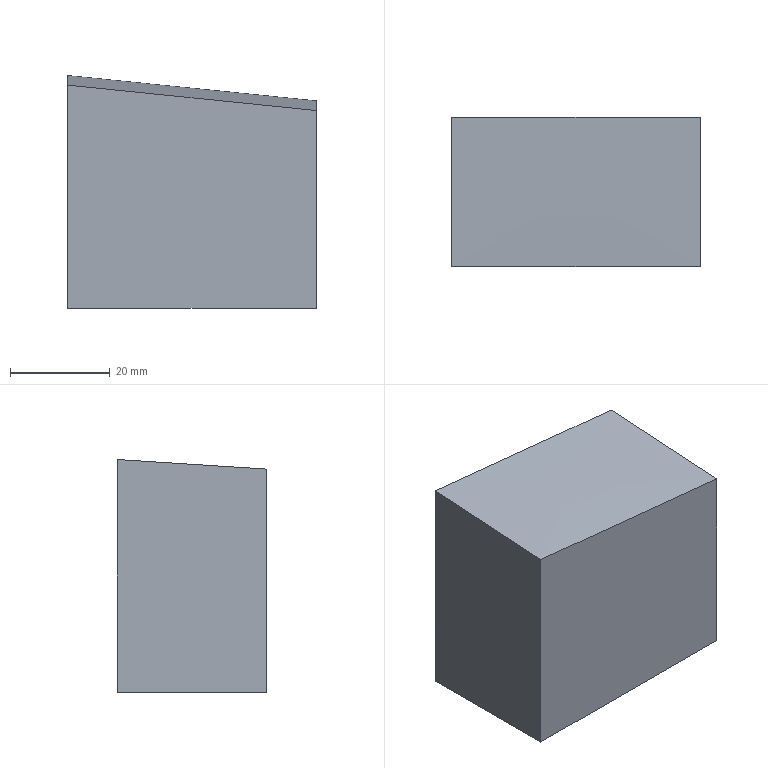Part | NX | features solid 2 | 1 solid | 6 faces | box 50 x 30 x 46.829 mm | volume 65041 mm3 | plane 5 | spline 1
STEP:
#1=CARTESIAN_POINT('',(437.5,-295.,54.902));
#2=VERTEX_POINT('',#1);
#3=CARTESIAN_POINT('',(487.5,-295.,49.786));
#4=VERTEX_POINT('',#3);
#5=CARTESIAN_POINT('',(437.5,-295.,54.902));
#6=CARTESIAN_POINT('',(454.172,-295.,53.249));
#7=CARTESIAN_POINT('',(470.839,-295.,51.542));
#8=CARTESIAN_POINT('',(487.5,-295.,49.786));
#9=B_SPLINE_CURVE_WITH_KNOTS('',3,(#5,#6,#7,#8),.UNSPECIFIED.,.F.,.F.,(4,4),(0.,0.05026),.UNSPECIFIED.);
#10=EDGE_CURVE('',#2,#4,#9,.T.);
#11=ORIENTED_EDGE('',*,*,#10,.F.);
#12=CARTESIAN_POINT('',(437.5,-295.,10.));
#13=VERTEX_POINT('',#12);
#14=CARTESIAN_POINT('',(437.5,-295.,210.));
#15=DIRECTION('',(0.,0.,-1.));
#16=VECTOR('',#15,1000.);
#17=LINE('',#14,#16);
#18=EDGE_CURVE('',#2,#13,#17,.T.);
#19=ORIENTED_EDGE('',*,*,#18,.T.);
#20=CARTESIAN_POINT('',(487.5,-295.,10.));
#21=VERTEX_POINT('',#20);
#22=CARTESIAN_POINT('',(437.5,-295.,10.));
#23=DIRECTION('',(1.,0.,0.));
#24=VECTOR('',#23,1000.);
#25=LINE('',#22,#24);
#26=EDGE_CURVE('',#13,#21,#25,.T.);
#27=ORIENTED_EDGE('',*,*,#26,.T.);
#28=CARTESIAN_POINT('',(487.5,-295.,210.));
#29=DIRECTION('',(0.,0.,-1.));
#30=VECTOR('',#29,1000.);
#31=LINE('',#28,#30);
#32=EDGE_CURVE('',#4,#21,#31,.T.);
#33=ORIENTED_EDGE('',*,*,#32,.F.);
#34=EDGE_LOOP('',(#11,#19,#27,#33));
#35=FACE_BOUND('',#34,.T.);
#36=CARTESIAN_POINT('',(437.5,-295.,210.));
#37=DIRECTION('',(0.,1.,0.));
#38=DIRECTION('',(0.,0.,1.));
#39=AXIS2_PLACEMENT_3D('',#36,#37,#38);
#40=PLANE('',#39);
#41=ADVANCED_FACE('',(#35),#40,.F.);
#42=ORIENTED_EDGE('',*,*,#18,.F.);
#43=CARTESIAN_POINT('',(437.5,-265.,56.829));
#44=VERTEX_POINT('',#43);
#45=CARTESIAN_POINT('',(437.5,-295.,54.902));
#46=CARTESIAN_POINT('',(437.5,-285.004,55.594));
#47=CARTESIAN_POINT('',(437.5,-275.003,56.235));
#48=CARTESIAN_POINT('',(437.5,-265.,56.829));
#49=B_SPLINE_CURVE_WITH_KNOTS('',3,(#45,#46,#47,#48),.UNSPECIFIED.,.F.,.F.,(4,4),(0.04695,0.07702),.UNSPECIFIED.);
#50=EDGE_CURVE('',#2,#44,#49,.T.);
#51=ORIENTED_EDGE('',*,*,#50,.T.);
#52=CARTESIAN_POINT('',(437.5,-265.,10.));
#53=VERTEX_POINT('',#52);
#54=CARTESIAN_POINT('',(437.5,-265.,210.));
#55=DIRECTION('',(0.,0.,-1.));
#56=VECTOR('',#55,1000.);
#57=LINE('',#54,#56);
#58=EDGE_CURVE('',#44,#53,#57,.T.);
#59=ORIENTED_EDGE('',*,*,#58,.T.);
#60=CARTESIAN_POINT('',(437.5,-515.,10.));
#61=DIRECTION('',(0.,-1.,0.));
#62=VECTOR('',#61,1000.);
#63=LINE('',#60,#62);
#64=EDGE_CURVE('',#13,#53,#63,.F.);
#65=ORIENTED_EDGE('',*,*,#64,.F.);
#66=EDGE_LOOP('',(#42,#51,#59,#65));
#67=FACE_BOUND('',#66,.T.);
#68=CARTESIAN_POINT('',(437.5,-515.,210.));
#69=DIRECTION('',(-1.,0.,0.));
#70=DIRECTION('',(0.,0.,1.));
#71=AXIS2_PLACEMENT_3D('',#68,#69,#70);
#72=PLANE('',#71);
#73=ADVANCED_FACE('',(#67),#72,.T.);
#74=ORIENTED_EDGE('',*,*,#58,.F.);
#75=CARTESIAN_POINT('',(487.5,-265.,51.724));
#76=VERTEX_POINT('',#75);
#77=CARTESIAN_POINT('',(437.5,-265.,56.829));
#78=CARTESIAN_POINT('',(454.171,-265.,55.18));
#79=CARTESIAN_POINT('',(470.839,-265.,53.476));
#80=CARTESIAN_POINT('',(487.5,-265.,51.724));
#81=B_SPLINE_CURVE_WITH_KNOTS('',3,(#77,#78,#79,#80),.UNSPECIFIED.,.F.,.F.,(4,4),(0.2849,0.3352),.UNSPECIFIED.);
#82=EDGE_CURVE('',#44,#76,#81,.T.);
#83=ORIENTED_EDGE('',*,*,#82,.T.);
#84=CARTESIAN_POINT('',(487.5,-265.,10.));
#85=VERTEX_POINT('',#84);
#86=CARTESIAN_POINT('',(487.5,-265.,210.));
#87=DIRECTION('',(0.,0.,-1.));
#88=VECTOR('',#87,1000.);
#89=LINE('',#86,#88);
#90=EDGE_CURVE('',#76,#85,#89,.T.);
#91=ORIENTED_EDGE('',*,*,#90,.T.);
#92=CARTESIAN_POINT('',(255.,-265.,10.));
#93=DIRECTION('',(-1.,0.,0.));
#94=VECTOR('',#93,1000.);
#95=LINE('',#92,#94);
#96=EDGE_CURVE('',#53,#85,#95,.F.);
#97=ORIENTED_EDGE('',*,*,#96,.F.);
#98=EDGE_LOOP('',(#74,#83,#91,#97));
#99=FACE_BOUND('',#98,.T.);
#100=CARTESIAN_POINT('',(255.,-265.,210.));
#101=DIRECTION('',(0.,1.,0.));
#102=DIRECTION('',(0.,0.,1.));
#103=AXIS2_PLACEMENT_3D('',#100,#101,#102);
#104=PLANE('',#103);
#105=ADVANCED_FACE('',(#99),#104,.T.);
#106=CARTESIAN_POINT('',(487.5,-295.,49.786));
#107=CARTESIAN_POINT('',(487.5,-285.005,50.482));
#108=CARTESIAN_POINT('',(487.5,-275.003,51.126));
#109=CARTESIAN_POINT('',(487.5,-265.,51.724));
#110=B_SPLINE_CURVE_WITH_KNOTS('',3,(#106,#107,#108,#109),.UNSPECIFIED.,.F.,.F.,(4,4),(0.1718,0.2018),.UNSPECIFIED.);
#111=EDGE_CURVE('',#4,#76,#110,.T.);
#112=ORIENTED_EDGE('',*,*,#111,.F.);
#113=ORIENTED_EDGE('',*,*,#32,.T.);
#114=CARTESIAN_POINT('',(487.5,-515.,10.));
#115=DIRECTION('',(0.,-1.,0.));
#116=VECTOR('',#115,1000.);
#117=LINE('',#114,#116);
#118=EDGE_CURVE('',#21,#85,#117,.F.);
#119=ORIENTED_EDGE('',*,*,#118,.T.);
#120=ORIENTED_EDGE('',*,*,#90,.F.);
#121=EDGE_LOOP('',(#112,#113,#119,#120));
#122=FACE_BOUND('',#121,.T.);
#123=CARTESIAN_POINT('',(487.5,-515.,210.));
#124=DIRECTION('',(-1.,0.,0.));
#125=DIRECTION('',(0.,0.,1.));
#126=AXIS2_PLACEMENT_3D('',#123,#124,#125);
#127=PLANE('',#126);
#128=ADVANCED_FACE('',(#122),#127,.F.);
#129=ORIENTED_EDGE('',*,*,#26,.F.);
#130=ORIENTED_EDGE('',*,*,#64,.T.);
#131=ORIENTED_EDGE('',*,*,#96,.T.);
#132=ORIENTED_EDGE('',*,*,#118,.F.);
#133=EDGE_LOOP('',(#129,#130,#131,#132));
#134=FACE_BOUND('',#133,.T.);
#135=CARTESIAN_POINT('',(255.,-515.,10.));
#136=DIRECTION('',(0.,0.,1.));
#137=DIRECTION('',(0.,1.,0.));
#138=AXIS2_PLACEMENT_3D('',#135,#136,#137);
#139=PLANE('',#138);
#140=ADVANCED_FACE('',(#134),#139,.F.);
#141=ORIENTED_EDGE('',*,*,#50,.F.);
#142=ORIENTED_EDGE('',*,*,#10,.T.);
#143=ORIENTED_EDGE('',*,*,#111,.T.);
#144=ORIENTED_EDGE('',*,*,#82,.F.);
#145=EDGE_LOOP('',(#141,#142,#143,#144));
#146=FACE_BOUND('',#145,.T.);
#147=CARTESIAN_POINT('',(437.198,-264.819,56.87));
#148=CARTESIAN_POINT('',(454.178,-264.817,55.191));
#149=CARTESIAN_POINT('',(471.069,-264.816,53.464));
#150=CARTESIAN_POINT('',(487.818,-264.815,51.702));
#151=CARTESIAN_POINT('',(437.191,-274.994,56.267));
#152=CARTESIAN_POINT('',(454.171,-274.993,54.587));
#153=CARTESIAN_POINT('',(471.062,-274.991,52.859));
#154=CARTESIAN_POINT('',(487.812,-274.99,51.095));
#155=CARTESIAN_POINT('',(437.184,-285.116,55.618));
#156=CARTESIAN_POINT('',(454.164,-285.114,53.937));
#157=CARTESIAN_POINT('',(471.055,-285.113,52.207));
#158=CARTESIAN_POINT('',(487.805,-285.111,50.442));
#159=CARTESIAN_POINT('',(437.176,-295.184,54.921));
#160=CARTESIAN_POINT('',(454.156,-295.182,53.239));
#161=CARTESIAN_POINT('',(471.048,-295.181,51.508));
#162=CARTESIAN_POINT('',(487.798,-295.179,49.742));
#163=B_SPLINE_SURFACE_WITH_KNOTS('',3,3,((#147,#148,#149,#150),(#151,#152,#153,#154),(#155,#156,#157,#158),(#159,#160,#161,#162)),.UNSPECIFIED.,.F.,.F.,.F.,(4,4),(4,4),(0.5343,0.5959),(0.7625,0.8244),.UNSPECIFIED.);
#164=ADVANCED_FACE('',(#146),#163,.T.);
#165=CLOSED_SHELL('',(#41,#73,#105,#128,#140,#164));
#166=MANIFOLD_SOLID_BREP('',#165);
#167=(LENGTH_UNIT()NAMED_UNIT(*)SI_UNIT(.MILLI.,.METRE.));
#168=UNCERTAINTY_MEASURE_WITH_UNIT(LENGTH_MEASURE(0.0508),#167,'','');
#169=(NAMED_UNIT(*)PLANE_ANGLE_UNIT()SI_UNIT($,.RADIAN.));
#170=(NAMED_UNIT(*)SI_UNIT($,.STERADIAN.)SOLID_ANGLE_UNIT());
#171=(GEOMETRIC_REPRESENTATION_CONTEXT(3)GLOBAL_UNCERTAINTY_ASSIGNED_CONTEXT((#168))GLOBAL_UNIT_ASSIGNED_CONTEXT((#167,#169,#170))REPRESENTATION_CONTEXT('',''));
#172=ADVANCED_BREP_SHAPE_REPRESENTATION('',(#166),#171);